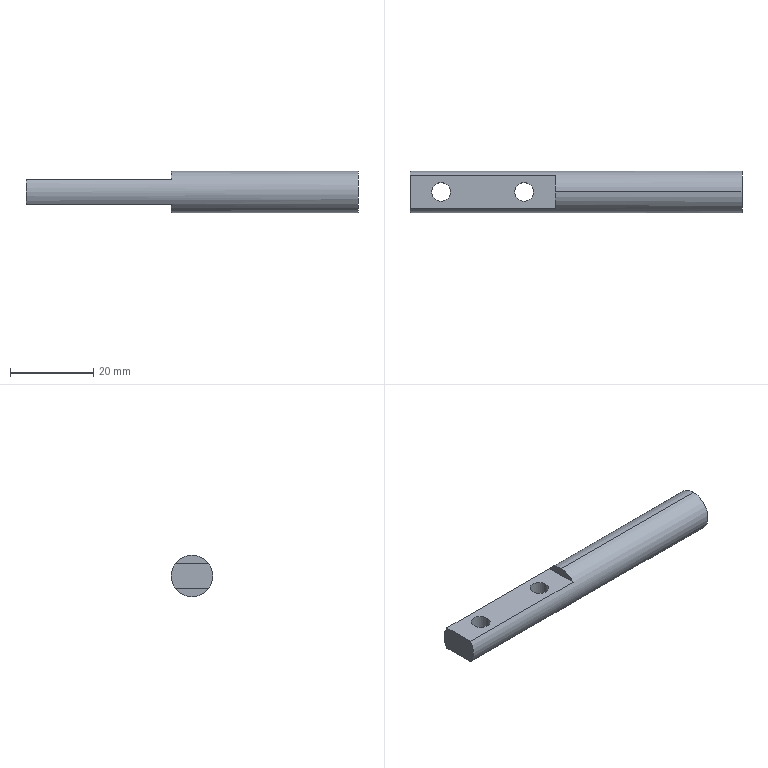Part | SolidWorks | features BaseBody 1 | 1 solid | 12 faces | box 80 x 10 x 10 mm | volume 5310 mm3 | cylinder 6 | plane 6 | commonest cylinder face diameters 4.5 x4 10 x2
STEP:
#1=CARTESIAN_POINT('',(5.25,0.,-3.));
#2=VERTEX_POINT('',#1);
#3=CARTESIAN_POINT('',(9.75,0.,-3.));
#4=VERTEX_POINT('',#3);
#5=CARTESIAN_POINT('',(7.5,0.,-3.));
#6=DIRECTION('',(0.,0.,1.));
#7=DIRECTION('',(0.,-1.,0.));
#8=AXIS2_PLACEMENT_3D('',#5,#6,#7);
#9=CIRCLE('',#8,2.25);
#10=EDGE_CURVE('',#2,#4,#9,.T.);
#11=ORIENTED_EDGE('',*,*,#10,.F.);
#12=CARTESIAN_POINT('',(5.25,0.,3.));
#13=VERTEX_POINT('',#12);
#14=CARTESIAN_POINT('',(5.25,0.,3.));
#15=DIRECTION('',(0.,0.,1.));
#16=VECTOR('',#15,1000.);
#17=LINE('',#14,#16);
#18=EDGE_CURVE('',#2,#13,#17,.T.);
#19=ORIENTED_EDGE('',*,*,#18,.T.);
#20=CARTESIAN_POINT('',(9.75,0.,3.));
#21=VERTEX_POINT('',#20);
#22=CARTESIAN_POINT('',(7.5,0.,3.));
#23=DIRECTION('',(0.,0.,1.));
#24=DIRECTION('',(1.,0.,0.));
#25=AXIS2_PLACEMENT_3D('',#22,#23,#24);
#26=CIRCLE('',#25,2.25);
#27=EDGE_CURVE('',#13,#21,#26,.T.);
#28=ORIENTED_EDGE('',*,*,#27,.T.);
#29=CARTESIAN_POINT('',(9.75,0.,3.));
#30=DIRECTION('',(0.,0.,1.));
#31=VECTOR('',#30,1000.);
#32=LINE('',#29,#31);
#33=EDGE_CURVE('',#4,#21,#32,.T.);
#34=ORIENTED_EDGE('',*,*,#33,.F.);
#35=EDGE_LOOP('',(#11,#19,#28,#34));
#36=FACE_OUTER_BOUND('',#35,.T.);
#37=CARTESIAN_POINT('',(7.5,0.,3.));
#38=DIRECTION('',(0.,0.,1.));
#39=DIRECTION('',(1.,0.,0.));
#40=AXIS2_PLACEMENT_3D('',#37,#38,#39);
#41=CYLINDRICAL_SURFACE('',#40,2.25);
#42=ADVANCED_FACE('',(#36),#41,.F.);
#43=CARTESIAN_POINT('',(25.25,0.,-3.));
#44=VERTEX_POINT('',#43);
#45=CARTESIAN_POINT('',(29.75,0.,-3.));
#46=VERTEX_POINT('',#45);
#47=CARTESIAN_POINT('',(27.5,0.,-3.));
#48=DIRECTION('',(0.,0.,1.));
#49=DIRECTION('',(0.,-1.,0.));
#50=AXIS2_PLACEMENT_3D('',#47,#48,#49);
#51=CIRCLE('',#50,2.25);
#52=EDGE_CURVE('',#44,#46,#51,.T.);
#53=ORIENTED_EDGE('',*,*,#52,.F.);
#54=CARTESIAN_POINT('',(25.25,0.,3.));
#55=VERTEX_POINT('',#54);
#56=CARTESIAN_POINT('',(25.25,0.,3.));
#57=DIRECTION('',(0.,0.,1.));
#58=VECTOR('',#57,1000.);
#59=LINE('',#56,#58);
#60=EDGE_CURVE('',#44,#55,#59,.T.);
#61=ORIENTED_EDGE('',*,*,#60,.T.);
#62=CARTESIAN_POINT('',(29.75,0.,3.));
#63=VERTEX_POINT('',#62);
#64=CARTESIAN_POINT('',(27.5,0.,3.));
#65=DIRECTION('',(0.,0.,1.));
#66=DIRECTION('',(1.,0.,0.));
#67=AXIS2_PLACEMENT_3D('',#64,#65,#66);
#68=CIRCLE('',#67,2.25);
#69=EDGE_CURVE('',#55,#63,#68,.T.);
#70=ORIENTED_EDGE('',*,*,#69,.T.);
#71=CARTESIAN_POINT('',(29.75,0.,3.));
#72=DIRECTION('',(0.,0.,1.));
#73=VECTOR('',#72,1000.);
#74=LINE('',#71,#73);
#75=EDGE_CURVE('',#46,#63,#74,.T.);
#76=ORIENTED_EDGE('',*,*,#75,.F.);
#77=EDGE_LOOP('',(#53,#61,#70,#76));
#78=FACE_OUTER_BOUND('',#77,.T.);
#79=CARTESIAN_POINT('',(27.5,0.,3.));
#80=DIRECTION('',(0.,0.,1.));
#81=DIRECTION('',(1.,0.,0.));
#82=AXIS2_PLACEMENT_3D('',#79,#80,#81);
#83=CYLINDRICAL_SURFACE('',#82,2.25);
#84=ADVANCED_FACE('',(#78),#83,.F.);
#85=CARTESIAN_POINT('',(80.,0.,-5.));
#86=VERTEX_POINT('',#85);
#87=CARTESIAN_POINT('',(80.,0.,5.));
#88=VERTEX_POINT('',#87);
#89=CARTESIAN_POINT('',(80.,0.,0.));
#90=DIRECTION('',(1.,0.,0.));
#91=DIRECTION('',(0.,0.,-1.));
#92=AXIS2_PLACEMENT_3D('',#89,#90,#91);
#93=CIRCLE('',#92,5.);
#94=EDGE_CURVE('',#86,#88,#93,.T.);
#95=ORIENTED_EDGE('',*,*,#94,.F.);
#96=CARTESIAN_POINT('',(35.,0.,-5.));
#97=VERTEX_POINT('',#96);
#98=CARTESIAN_POINT('',(80.,0.,-5.));
#99=DIRECTION('',(-1.,0.,0.));
#100=VECTOR('',#99,1000.);
#101=LINE('',#98,#100);
#102=EDGE_CURVE('',#86,#97,#101,.T.);
#103=ORIENTED_EDGE('',*,*,#102,.T.);
#104=CARTESIAN_POINT('',(35.,4.,-3.));
#105=VERTEX_POINT('',#104);
#106=CARTESIAN_POINT('',(35.,0.,0.));
#107=DIRECTION('',(-1.,0.,0.));
#108=DIRECTION('',(0.,0.,1.));
#109=AXIS2_PLACEMENT_3D('',#106,#107,#108);
#110=CIRCLE('',#109,5.);
#111=EDGE_CURVE('',#105,#97,#110,.T.);
#112=ORIENTED_EDGE('',*,*,#111,.F.);
#113=CARTESIAN_POINT('',(0.,4.,-3.));
#114=VERTEX_POINT('',#113);
#115=CARTESIAN_POINT('',(80.,4.,-3.));
#116=DIRECTION('',(-1.,0.,0.));
#117=VECTOR('',#116,1000.);
#118=LINE('',#115,#117);
#119=EDGE_CURVE('',#105,#114,#118,.T.);
#120=ORIENTED_EDGE('',*,*,#119,.T.);
#121=CARTESIAN_POINT('',(0.,4.,3.));
#122=VERTEX_POINT('',#121);
#123=CARTESIAN_POINT('',(0.,0.,0.));
#124=DIRECTION('',(1.,0.,0.));
#125=DIRECTION('',(0.,0.,-1.));
#126=AXIS2_PLACEMENT_3D('',#123,#124,#125);
#127=CIRCLE('',#126,5.);
#128=EDGE_CURVE('',#114,#122,#127,.T.);
#129=ORIENTED_EDGE('',*,*,#128,.T.);
#130=CARTESIAN_POINT('',(35.,4.,3.));
#131=VERTEX_POINT('',#130);
#132=CARTESIAN_POINT('',(80.,4.,3.));
#133=DIRECTION('',(1.,0.,0.));
#134=VECTOR('',#133,1000.);
#135=LINE('',#132,#134);
#136=EDGE_CURVE('',#122,#131,#135,.T.);
#137=ORIENTED_EDGE('',*,*,#136,.T.);
#138=CARTESIAN_POINT('',(35.,0.,5.));
#139=VERTEX_POINT('',#138);
#140=CARTESIAN_POINT('',(35.,0.,0.));
#141=DIRECTION('',(-1.,0.,0.));
#142=DIRECTION('',(0.,0.,1.));
#143=AXIS2_PLACEMENT_3D('',#140,#141,#142);
#144=CIRCLE('',#143,5.);
#145=EDGE_CURVE('',#139,#131,#144,.T.);
#146=ORIENTED_EDGE('',*,*,#145,.F.);
#147=CARTESIAN_POINT('',(80.,0.,5.));
#148=DIRECTION('',(-1.,0.,0.));
#149=VECTOR('',#148,1000.);
#150=LINE('',#147,#149);
#151=EDGE_CURVE('',#88,#139,#150,.T.);
#152=ORIENTED_EDGE('',*,*,#151,.F.);
#153=EDGE_LOOP('',(#95,#103,#112,#120,#129,#137,#146,#152));
#154=FACE_OUTER_BOUND('',#153,.T.);
#155=CARTESIAN_POINT('',(80.,0.,0.));
#156=DIRECTION('',(-1.,0.,0.));
#157=DIRECTION('',(0.,0.,1.));
#158=AXIS2_PLACEMENT_3D('',#155,#156,#157);
#159=CYLINDRICAL_SURFACE('',#158,5.);
#160=ADVANCED_FACE('',(#154),#159,.T.);
#161=ORIENTED_EDGE('',*,*,#102,.F.);
#162=CARTESIAN_POINT('',(80.,0.,0.));
#163=DIRECTION('',(1.,0.,0.));
#164=DIRECTION('',(0.,0.,-1.));
#165=AXIS2_PLACEMENT_3D('',#162,#163,#164);
#166=CIRCLE('',#165,5.);
#167=EDGE_CURVE('',#88,#86,#166,.T.);
#168=ORIENTED_EDGE('',*,*,#167,.F.);
#169=ORIENTED_EDGE('',*,*,#151,.T.);
#170=CARTESIAN_POINT('',(35.,-4.,3.));
#171=VERTEX_POINT('',#170);
#172=CARTESIAN_POINT('',(35.,0.,0.));
#173=DIRECTION('',(-1.,0.,0.));
#174=DIRECTION('',(0.,0.,1.));
#175=AXIS2_PLACEMENT_3D('',#172,#173,#174);
#176=CIRCLE('',#175,5.);
#177=EDGE_CURVE('',#171,#139,#176,.T.);
#178=ORIENTED_EDGE('',*,*,#177,.F.);
#179=CARTESIAN_POINT('',(0.,-4.,3.));
#180=VERTEX_POINT('',#179);
#181=CARTESIAN_POINT('',(80.,-4.,3.));
#182=DIRECTION('',(-1.,0.,0.));
#183=VECTOR('',#182,1000.);
#184=LINE('',#181,#183);
#185=EDGE_CURVE('',#171,#180,#184,.T.);
#186=ORIENTED_EDGE('',*,*,#185,.T.);
#187=CARTESIAN_POINT('',(0.,-4.,-3.));
#188=VERTEX_POINT('',#187);
#189=CARTESIAN_POINT('',(0.,0.,0.));
#190=DIRECTION('',(1.,0.,0.));
#191=DIRECTION('',(0.,0.,-1.));
#192=AXIS2_PLACEMENT_3D('',#189,#190,#191);
#193=CIRCLE('',#192,5.);
#194=EDGE_CURVE('',#180,#188,#193,.T.);
#195=ORIENTED_EDGE('',*,*,#194,.T.);
#196=CARTESIAN_POINT('',(35.,-4.,-3.));
#197=VERTEX_POINT('',#196);
#198=CARTESIAN_POINT('',(80.,-4.,-3.));
#199=DIRECTION('',(1.,0.,0.));
#200=VECTOR('',#199,1000.);
#201=LINE('',#198,#200);
#202=EDGE_CURVE('',#188,#197,#201,.T.);
#203=ORIENTED_EDGE('',*,*,#202,.T.);
#204=CARTESIAN_POINT('',(35.,0.,0.));
#205=DIRECTION('',(-1.,0.,0.));
#206=DIRECTION('',(0.,0.,1.));
#207=AXIS2_PLACEMENT_3D('',#204,#205,#206);
#208=CIRCLE('',#207,5.);
#209=EDGE_CURVE('',#97,#197,#208,.T.);
#210=ORIENTED_EDGE('',*,*,#209,.F.);
#211=EDGE_LOOP('',(#161,#168,#169,#178,#186,#195,#203,#210));
#212=FACE_OUTER_BOUND('',#211,.T.);
#213=CARTESIAN_POINT('',(80.,0.,0.));
#214=DIRECTION('',(-1.,0.,0.));
#215=DIRECTION('',(0.,0.,1.));
#216=AXIS2_PLACEMENT_3D('',#213,#214,#215);
#217=CYLINDRICAL_SURFACE('',#216,5.);
#218=ADVANCED_FACE('',(#212),#217,.T.);
#219=ORIENTED_EDGE('',*,*,#167,.T.);
#220=ORIENTED_EDGE('',*,*,#94,.T.);
#221=EDGE_LOOP('',(#219,#220));
#222=FACE_OUTER_BOUND('',#221,.T.);
#223=CARTESIAN_POINT('',(80.,0.,0.));
#224=DIRECTION('',(1.,0.,0.));
#225=DIRECTION('',(0.,0.,-1.));
#226=AXIS2_PLACEMENT_3D('',#223,#224,#225);
#227=PLANE('',#226);
#228=ADVANCED_FACE('',(#222),#227,.T.);
#229=ORIENTED_EDGE('',*,*,#194,.F.);
#230=CARTESIAN_POINT('',(0.,0.,3.));
#231=DIRECTION('',(0.,1.,0.));
#232=VECTOR('',#231,1000.);
#233=LINE('',#230,#232);
#234=EDGE_CURVE('',#180,#122,#233,.T.);
#235=ORIENTED_EDGE('',*,*,#234,.T.);
#236=ORIENTED_EDGE('',*,*,#128,.F.);
#237=CARTESIAN_POINT('',(0.,0.,-3.));
#238=DIRECTION('',(0.,-1.,0.));
#239=VECTOR('',#238,1000.);
#240=LINE('',#237,#239);
#241=EDGE_CURVE('',#114,#188,#240,.T.);
#242=ORIENTED_EDGE('',*,*,#241,.T.);
#243=EDGE_LOOP('',(#229,#235,#236,#242));
#244=FACE_OUTER_BOUND('',#243,.T.);
#245=CARTESIAN_POINT('',(0.,0.,0.));
#246=DIRECTION('',(1.,0.,0.));
#247=DIRECTION('',(0.,0.,-1.));
#248=AXIS2_PLACEMENT_3D('',#245,#246,#247);
#249=PLANE('',#248);
#250=ADVANCED_FACE('',(#244),#249,.F.);
#251=ORIENTED_EDGE('',*,*,#111,.T.);
#252=ORIENTED_EDGE('',*,*,#209,.T.);
#253=CARTESIAN_POINT('',(35.,5.,-3.));
#254=DIRECTION('',(0.,1.,0.));
#255=VECTOR('',#254,1000.);
#256=LINE('',#253,#255);
#257=EDGE_CURVE('',#197,#105,#256,.T.);
#258=ORIENTED_EDGE('',*,*,#257,.T.);
#259=EDGE_LOOP('',(#251,#252,#258));
#260=FACE_OUTER_BOUND('',#259,.T.);
#261=CARTESIAN_POINT('',(35.,0.,0.));
#262=DIRECTION('',(-1.,0.,0.));
#263=DIRECTION('',(0.,0.,1.));
#264=AXIS2_PLACEMENT_3D('',#261,#262,#263);
#265=PLANE('',#264);
#266=ADVANCED_FACE('',(#260),#265,.T.);
#267=CARTESIAN_POINT('',(7.5,0.,-3.));
#268=DIRECTION('',(0.,0.,1.));
#269=DIRECTION('',(0.,-1.,0.));
#270=AXIS2_PLACEMENT_3D('',#267,#268,#269);
#271=CIRCLE('',#270,2.25);
#272=EDGE_CURVE('',#4,#2,#271,.T.);
#273=ORIENTED_EDGE('',*,*,#272,.T.);
#274=ORIENTED_EDGE('',*,*,#10,.T.);
#275=EDGE_LOOP('',(#273,#274));
#276=FACE_BOUND('',#275,.T.);
#277=CARTESIAN_POINT('',(27.5,0.,-3.));
#278=DIRECTION('',(0.,0.,1.));
#279=DIRECTION('',(0.,-1.,0.));
#280=AXIS2_PLACEMENT_3D('',#277,#278,#279);
#281=CIRCLE('',#280,2.25);
#282=EDGE_CURVE('',#46,#44,#281,.T.);
#283=ORIENTED_EDGE('',*,*,#282,.T.);
#284=ORIENTED_EDGE('',*,*,#52,.T.);
#285=EDGE_LOOP('',(#283,#284));
#286=FACE_BOUND('',#285,.T.);
#287=ORIENTED_EDGE('',*,*,#257,.F.);
#288=ORIENTED_EDGE('',*,*,#202,.F.);
#289=ORIENTED_EDGE('',*,*,#241,.F.);
#290=ORIENTED_EDGE('',*,*,#119,.F.);
#291=EDGE_LOOP('',(#287,#288,#289,#290));
#292=FACE_OUTER_BOUND('',#291,.T.);
#293=CARTESIAN_POINT('',(35.,5.,-3.));
#294=DIRECTION('',(0.,0.,1.));
#295=DIRECTION('',(0.,-1.,0.));
#296=AXIS2_PLACEMENT_3D('',#293,#294,#295);
#297=PLANE('',#296);
#298=ADVANCED_FACE('',(#276,#286,#292),#297,.F.);
#299=ORIENTED_EDGE('',*,*,#177,.T.);
#300=ORIENTED_EDGE('',*,*,#145,.T.);
#301=CARTESIAN_POINT('',(35.,5.,3.));
#302=DIRECTION('',(0.,-1.,0.));
#303=VECTOR('',#302,1000.);
#304=LINE('',#301,#303);
#305=EDGE_CURVE('',#131,#171,#304,.T.);
#306=ORIENTED_EDGE('',*,*,#305,.T.);
#307=EDGE_LOOP('',(#299,#300,#306));
#308=FACE_OUTER_BOUND('',#307,.T.);
#309=CARTESIAN_POINT('',(35.,0.,0.));
#310=DIRECTION('',(-1.,0.,0.));
#311=DIRECTION('',(0.,0.,1.));
#312=AXIS2_PLACEMENT_3D('',#309,#310,#311);
#313=PLANE('',#312);
#314=ADVANCED_FACE('',(#308),#313,.T.);
#315=CARTESIAN_POINT('',(7.5,0.,3.));
#316=DIRECTION('',(0.,0.,1.));
#317=DIRECTION('',(1.,0.,0.));
#318=AXIS2_PLACEMENT_3D('',#315,#316,#317);
#319=CIRCLE('',#318,2.25);
#320=EDGE_CURVE('',#21,#13,#319,.T.);
#321=ORIENTED_EDGE('',*,*,#320,.F.);
#322=ORIENTED_EDGE('',*,*,#27,.F.);
#323=EDGE_LOOP('',(#321,#322));
#324=FACE_BOUND('',#323,.T.);
#325=CARTESIAN_POINT('',(27.5,0.,3.));
#326=DIRECTION('',(0.,0.,1.));
#327=DIRECTION('',(1.,0.,0.));
#328=AXIS2_PLACEMENT_3D('',#325,#326,#327);
#329=CIRCLE('',#328,2.25);
#330=EDGE_CURVE('',#63,#55,#329,.T.);
#331=ORIENTED_EDGE('',*,*,#330,.F.);
#332=ORIENTED_EDGE('',*,*,#69,.F.);
#333=EDGE_LOOP('',(#331,#332));
#334=FACE_BOUND('',#333,.T.);
#335=ORIENTED_EDGE('',*,*,#305,.F.);
#336=ORIENTED_EDGE('',*,*,#136,.F.);
#337=ORIENTED_EDGE('',*,*,#234,.F.);
#338=ORIENTED_EDGE('',*,*,#185,.F.);
#339=EDGE_LOOP('',(#335,#336,#337,#338));
#340=FACE_OUTER_BOUND('',#339,.T.);
#341=CARTESIAN_POINT('',(35.,5.,3.));
#342=DIRECTION('',(0.,0.,-1.));
#343=DIRECTION('',(0.,1.,0.));
#344=AXIS2_PLACEMENT_3D('',#341,#342,#343);
#345=PLANE('',#344);
#346=ADVANCED_FACE('',(#324,#334,#340),#345,.F.);
#347=ORIENTED_EDGE('',*,*,#60,.F.);
#348=ORIENTED_EDGE('',*,*,#282,.F.);
#349=ORIENTED_EDGE('',*,*,#75,.T.);
#350=ORIENTED_EDGE('',*,*,#330,.T.);
#351=EDGE_LOOP('',(#347,#348,#349,#350));
#352=FACE_OUTER_BOUND('',#351,.T.);
#353=CARTESIAN_POINT('',(27.5,0.,3.));
#354=DIRECTION('',(0.,0.,1.));
#355=DIRECTION('',(1.,0.,0.));
#356=AXIS2_PLACEMENT_3D('',#353,#354,#355);
#357=CYLINDRICAL_SURFACE('',#356,2.25);
#358=ADVANCED_FACE('',(#352),#357,.F.);
#359=ORIENTED_EDGE('',*,*,#18,.F.);
#360=ORIENTED_EDGE('',*,*,#272,.F.);
#361=ORIENTED_EDGE('',*,*,#33,.T.);
#362=ORIENTED_EDGE('',*,*,#320,.T.);
#363=EDGE_LOOP('',(#359,#360,#361,#362));
#364=FACE_OUTER_BOUND('',#363,.T.);
#365=CARTESIAN_POINT('',(7.5,0.,3.));
#366=DIRECTION('',(0.,0.,1.));
#367=DIRECTION('',(1.,0.,0.));
#368=AXIS2_PLACEMENT_3D('',#365,#366,#367);
#369=CYLINDRICAL_SURFACE('',#368,2.25);
#370=ADVANCED_FACE('',(#364),#369,.F.);
#371=CLOSED_SHELL('',(#42,#84,#160,#218,#228,#250,#266,#298,#314,#346,#358,#370));
#372=MANIFOLD_SOLID_BREP('',#371);
#373=CARTESIAN_POINT('',(0.,0.,0.));
#374=DIRECTION('',(0.,0.,1.));
#375=DIRECTION('',(1.,0.,0.));
#376=AXIS2_PLACEMENT_3D('',#373,#374,#375);
#377=(LENGTH_UNIT()NAMED_UNIT(*)SI_UNIT(.MILLI.,.METRE.));
#378=UNCERTAINTY_MEASURE_WITH_UNIT(LENGTH_MEASURE(0.00001),#377,'','');
#379=(NAMED_UNIT(*)PLANE_ANGLE_UNIT()SI_UNIT($,.RADIAN.));
#380=(NAMED_UNIT(*)SI_UNIT($,.STERADIAN.)SOLID_ANGLE_UNIT());
#381=(GEOMETRIC_REPRESENTATION_CONTEXT(3)GLOBAL_UNCERTAINTY_ASSIGNED_CONTEXT((#378))GLOBAL_UNIT_ASSIGNED_CONTEXT((#377,#379,#380))REPRESENTATION_CONTEXT('',''));
#382=ADVANCED_BREP_SHAPE_REPRESENTATION('',(#372,#376),#381);